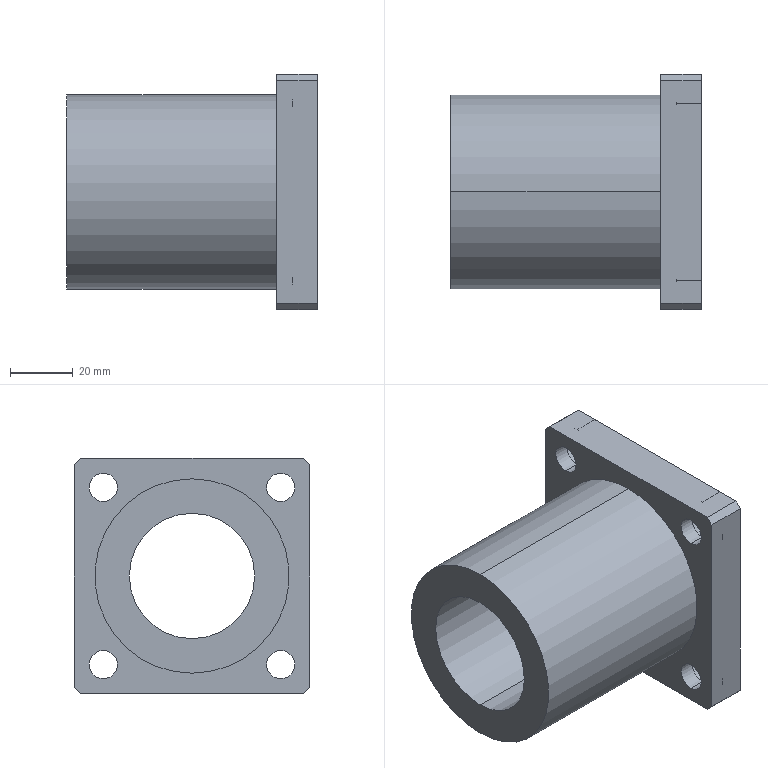Part | SolidWorks | features Chamfer 1, Extrusion 1, HoleWzd 1, ICE 1 | 1 solid | 35 faces | box 80 x 75 x 75 mm | volume 165352 mm3 | cylinder 20 | plane 15 | commonest cylinder face diameters 9 x8 18 x8 40 x2 62 x2
STEP:
#1=CARTESIAN_POINT('',(72.,28.284,-19.284));
#2=VERTEX_POINT('',#1);
#3=CARTESIAN_POINT('',(72.,28.284,-37.284));
#4=VERTEX_POINT('',#3);
#5=CARTESIAN_POINT('',(72.,28.284,-28.284));
#6=DIRECTION('',(1.,0.,0.));
#7=DIRECTION('',(0.,0.,-1.));
#8=AXIS2_PLACEMENT_3D('',#5,#6,#7);
#9=CIRCLE('',#8,9.);
#10=EDGE_CURVE('',#2,#4,#9,.T.);
#11=ORIENTED_EDGE('',*,*,#10,.F.);
#12=CARTESIAN_POINT('',(80.,28.284,-19.284));
#13=VERTEX_POINT('',#12);
#14=CARTESIAN_POINT('',(80.,28.284,-19.284));
#15=DIRECTION('',(1.,0.,0.));
#16=VECTOR('',#15,1000.);
#17=LINE('',#14,#16);
#18=EDGE_CURVE('',#2,#13,#17,.T.);
#19=ORIENTED_EDGE('',*,*,#18,.T.);
#20=CARTESIAN_POINT('',(80.,28.284,-37.284));
#21=VERTEX_POINT('',#20);
#22=CARTESIAN_POINT('',(80.,28.284,-28.284));
#23=DIRECTION('',(1.,0.,0.));
#24=DIRECTION('',(0.,0.,-1.));
#25=AXIS2_PLACEMENT_3D('',#22,#23,#24);
#26=CIRCLE('',#25,9.);
#27=EDGE_CURVE('',#13,#21,#26,.T.);
#28=ORIENTED_EDGE('',*,*,#27,.T.);
#29=CARTESIAN_POINT('',(80.,28.284,-37.284));
#30=DIRECTION('',(1.,0.,0.));
#31=VECTOR('',#30,1000.);
#32=LINE('',#29,#31);
#33=EDGE_CURVE('',#4,#21,#32,.T.);
#34=ORIENTED_EDGE('',*,*,#33,.F.);
#35=EDGE_LOOP('',(#11,#19,#28,#34));
#36=FACE_OUTER_BOUND('',#35,.T.);
#37=CARTESIAN_POINT('',(80.,28.284,-28.284));
#38=DIRECTION('',(1.,0.,0.));
#39=DIRECTION('',(0.,0.,-1.));
#40=AXIS2_PLACEMENT_3D('',#37,#38,#39);
#41=CYLINDRICAL_SURFACE('',#40,9.);
#42=ADVANCED_FACE('',(#36),#41,.F.);
#43=CARTESIAN_POINT('',(67.,28.284,-23.784));
#44=VERTEX_POINT('',#43);
#45=CARTESIAN_POINT('',(67.,28.284,-32.784));
#46=VERTEX_POINT('',#45);
#47=CARTESIAN_POINT('',(67.,28.284,-28.284));
#48=DIRECTION('',(1.,0.,0.));
#49=DIRECTION('',(0.,0.,-1.));
#50=AXIS2_PLACEMENT_3D('',#47,#48,#49);
#51=CIRCLE('',#50,4.5);
#52=EDGE_CURVE('',#44,#46,#51,.T.);
#53=ORIENTED_EDGE('',*,*,#52,.F.);
#54=CARTESIAN_POINT('',(72.,28.284,-23.784));
#55=VERTEX_POINT('',#54);
#56=CARTESIAN_POINT('',(80.,28.284,-23.784));
#57=DIRECTION('',(1.,0.,0.));
#58=VECTOR('',#57,1000.);
#59=LINE('',#56,#58);
#60=EDGE_CURVE('',#44,#55,#59,.T.);
#61=ORIENTED_EDGE('',*,*,#60,.T.);
#62=CARTESIAN_POINT('',(72.,28.284,-32.784));
#63=VERTEX_POINT('',#62);
#64=CARTESIAN_POINT('',(72.,28.284,-28.284));
#65=DIRECTION('',(1.,0.,0.));
#66=DIRECTION('',(0.,0.,-1.));
#67=AXIS2_PLACEMENT_3D('',#64,#65,#66);
#68=CIRCLE('',#67,4.5);
#69=EDGE_CURVE('',#55,#63,#68,.T.);
#70=ORIENTED_EDGE('',*,*,#69,.T.);
#71=CARTESIAN_POINT('',(80.,28.284,-32.784));
#72=DIRECTION('',(1.,0.,0.));
#73=VECTOR('',#72,1000.);
#74=LINE('',#71,#73);
#75=EDGE_CURVE('',#46,#63,#74,.T.);
#76=ORIENTED_EDGE('',*,*,#75,.F.);
#77=EDGE_LOOP('',(#53,#61,#70,#76));
#78=FACE_OUTER_BOUND('',#77,.T.);
#79=CARTESIAN_POINT('',(80.,28.284,-28.284));
#80=DIRECTION('',(1.,0.,0.));
#81=DIRECTION('',(0.,0.,-1.));
#82=AXIS2_PLACEMENT_3D('',#79,#80,#81);
#83=CYLINDRICAL_SURFACE('',#82,4.5);
#84=ADVANCED_FACE('',(#78),#83,.F.);
#85=CARTESIAN_POINT('',(72.,-28.284,-19.284));
#86=VERTEX_POINT('',#85);
#87=CARTESIAN_POINT('',(72.,-28.284,-37.284));
#88=VERTEX_POINT('',#87);
#89=CARTESIAN_POINT('',(72.,-28.284,-28.284));
#90=DIRECTION('',(1.,0.,0.));
#91=DIRECTION('',(0.,0.,-1.));
#92=AXIS2_PLACEMENT_3D('',#89,#90,#91);
#93=CIRCLE('',#92,9.);
#94=EDGE_CURVE('',#86,#88,#93,.T.);
#95=ORIENTED_EDGE('',*,*,#94,.F.);
#96=CARTESIAN_POINT('',(80.,-28.284,-19.284));
#97=VERTEX_POINT('',#96);
#98=CARTESIAN_POINT('',(80.,-28.284,-19.284));
#99=DIRECTION('',(1.,0.,0.));
#100=VECTOR('',#99,1000.);
#101=LINE('',#98,#100);
#102=EDGE_CURVE('',#86,#97,#101,.T.);
#103=ORIENTED_EDGE('',*,*,#102,.T.);
#104=CARTESIAN_POINT('',(80.,-28.284,-37.284));
#105=VERTEX_POINT('',#104);
#106=CARTESIAN_POINT('',(80.,-28.284,-28.284));
#107=DIRECTION('',(1.,0.,0.));
#108=DIRECTION('',(0.,0.,-1.));
#109=AXIS2_PLACEMENT_3D('',#106,#107,#108);
#110=CIRCLE('',#109,9.);
#111=EDGE_CURVE('',#97,#105,#110,.T.);
#112=ORIENTED_EDGE('',*,*,#111,.T.);
#113=CARTESIAN_POINT('',(80.,-28.284,-37.284));
#114=DIRECTION('',(1.,0.,0.));
#115=VECTOR('',#114,1000.);
#116=LINE('',#113,#115);
#117=EDGE_CURVE('',#88,#105,#116,.T.);
#118=ORIENTED_EDGE('',*,*,#117,.F.);
#119=EDGE_LOOP('',(#95,#103,#112,#118));
#120=FACE_OUTER_BOUND('',#119,.T.);
#121=CARTESIAN_POINT('',(80.,-28.284,-28.284));
#122=DIRECTION('',(1.,0.,0.));
#123=DIRECTION('',(0.,0.,-1.));
#124=AXIS2_PLACEMENT_3D('',#121,#122,#123);
#125=CYLINDRICAL_SURFACE('',#124,9.);
#126=ADVANCED_FACE('',(#120),#125,.F.);
#127=CARTESIAN_POINT('',(67.,-28.284,-23.784));
#128=VERTEX_POINT('',#127);
#129=CARTESIAN_POINT('',(67.,-28.284,-32.784));
#130=VERTEX_POINT('',#129);
#131=CARTESIAN_POINT('',(67.,-28.284,-28.284));
#132=DIRECTION('',(1.,0.,0.));
#133=DIRECTION('',(0.,0.,-1.));
#134=AXIS2_PLACEMENT_3D('',#131,#132,#133);
#135=CIRCLE('',#134,4.5);
#136=EDGE_CURVE('',#128,#130,#135,.T.);
#137=ORIENTED_EDGE('',*,*,#136,.F.);
#138=CARTESIAN_POINT('',(72.,-28.284,-23.784));
#139=VERTEX_POINT('',#138);
#140=CARTESIAN_POINT('',(80.,-28.284,-23.784));
#141=DIRECTION('',(1.,0.,0.));
#142=VECTOR('',#141,1000.);
#143=LINE('',#140,#142);
#144=EDGE_CURVE('',#128,#139,#143,.T.);
#145=ORIENTED_EDGE('',*,*,#144,.T.);
#146=CARTESIAN_POINT('',(72.,-28.284,-32.784));
#147=VERTEX_POINT('',#146);
#148=CARTESIAN_POINT('',(72.,-28.284,-28.284));
#149=DIRECTION('',(1.,0.,0.));
#150=DIRECTION('',(0.,0.,-1.));
#151=AXIS2_PLACEMENT_3D('',#148,#149,#150);
#152=CIRCLE('',#151,4.5);
#153=EDGE_CURVE('',#139,#147,#152,.T.);
#154=ORIENTED_EDGE('',*,*,#153,.T.);
#155=CARTESIAN_POINT('',(80.,-28.284,-32.784));
#156=DIRECTION('',(1.,0.,0.));
#157=VECTOR('',#156,1000.);
#158=LINE('',#155,#157);
#159=EDGE_CURVE('',#130,#147,#158,.T.);
#160=ORIENTED_EDGE('',*,*,#159,.F.);
#161=EDGE_LOOP('',(#137,#145,#154,#160));
#162=FACE_OUTER_BOUND('',#161,.T.);
#163=CARTESIAN_POINT('',(80.,-28.284,-28.284));
#164=DIRECTION('',(1.,0.,0.));
#165=DIRECTION('',(0.,0.,-1.));
#166=AXIS2_PLACEMENT_3D('',#163,#164,#165);
#167=CYLINDRICAL_SURFACE('',#166,4.5);
#168=ADVANCED_FACE('',(#162),#167,.F.);
#169=CARTESIAN_POINT('',(72.,-28.284,37.284));
#170=VERTEX_POINT('',#169);
#171=CARTESIAN_POINT('',(72.,-28.284,19.284));
#172=VERTEX_POINT('',#171);
#173=CARTESIAN_POINT('',(72.,-28.284,28.284));
#174=DIRECTION('',(1.,0.,0.));
#175=DIRECTION('',(0.,0.,-1.));
#176=AXIS2_PLACEMENT_3D('',#173,#174,#175);
#177=CIRCLE('',#176,9.);
#178=EDGE_CURVE('',#170,#172,#177,.T.);
#179=ORIENTED_EDGE('',*,*,#178,.F.);
#180=CARTESIAN_POINT('',(80.,-28.284,37.284));
#181=VERTEX_POINT('',#180);
#182=CARTESIAN_POINT('',(80.,-28.284,37.284));
#183=DIRECTION('',(1.,0.,0.));
#184=VECTOR('',#183,1000.);
#185=LINE('',#182,#184);
#186=EDGE_CURVE('',#170,#181,#185,.T.);
#187=ORIENTED_EDGE('',*,*,#186,.T.);
#188=CARTESIAN_POINT('',(80.,-28.284,19.284));
#189=VERTEX_POINT('',#188);
#190=CARTESIAN_POINT('',(80.,-28.284,28.284));
#191=DIRECTION('',(1.,0.,0.));
#192=DIRECTION('',(0.,0.,-1.));
#193=AXIS2_PLACEMENT_3D('',#190,#191,#192);
#194=CIRCLE('',#193,9.);
#195=EDGE_CURVE('',#181,#189,#194,.T.);
#196=ORIENTED_EDGE('',*,*,#195,.T.);
#197=CARTESIAN_POINT('',(80.,-28.284,19.284));
#198=DIRECTION('',(1.,0.,0.));
#199=VECTOR('',#198,1000.);
#200=LINE('',#197,#199);
#201=EDGE_CURVE('',#172,#189,#200,.T.);
#202=ORIENTED_EDGE('',*,*,#201,.F.);
#203=EDGE_LOOP('',(#179,#187,#196,#202));
#204=FACE_OUTER_BOUND('',#203,.T.);
#205=CARTESIAN_POINT('',(80.,-28.284,28.284));
#206=DIRECTION('',(1.,0.,0.));
#207=DIRECTION('',(0.,0.,-1.));
#208=AXIS2_PLACEMENT_3D('',#205,#206,#207);
#209=CYLINDRICAL_SURFACE('',#208,9.);
#210=ADVANCED_FACE('',(#204),#209,.F.);
#211=CARTESIAN_POINT('',(67.,-28.284,32.784));
#212=VERTEX_POINT('',#211);
#213=CARTESIAN_POINT('',(67.,-28.284,23.784));
#214=VERTEX_POINT('',#213);
#215=CARTESIAN_POINT('',(67.,-28.284,28.284));
#216=DIRECTION('',(1.,0.,0.));
#217=DIRECTION('',(0.,0.,-1.));
#218=AXIS2_PLACEMENT_3D('',#215,#216,#217);
#219=CIRCLE('',#218,4.5);
#220=EDGE_CURVE('',#212,#214,#219,.T.);
#221=ORIENTED_EDGE('',*,*,#220,.F.);
#222=CARTESIAN_POINT('',(72.,-28.284,32.784));
#223=VERTEX_POINT('',#222);
#224=CARTESIAN_POINT('',(80.,-28.284,32.784));
#225=DIRECTION('',(1.,0.,0.));
#226=VECTOR('',#225,1000.);
#227=LINE('',#224,#226);
#228=EDGE_CURVE('',#212,#223,#227,.T.);
#229=ORIENTED_EDGE('',*,*,#228,.T.);
#230=CARTESIAN_POINT('',(72.,-28.284,23.784));
#231=VERTEX_POINT('',#230);
#232=CARTESIAN_POINT('',(72.,-28.284,28.284));
#233=DIRECTION('',(1.,0.,0.));
#234=DIRECTION('',(0.,0.,-1.));
#235=AXIS2_PLACEMENT_3D('',#232,#233,#234);
#236=CIRCLE('',#235,4.5);
#237=EDGE_CURVE('',#223,#231,#236,.T.);
#238=ORIENTED_EDGE('',*,*,#237,.T.);
#239=CARTESIAN_POINT('',(80.,-28.284,23.784));
#240=DIRECTION('',(1.,0.,0.));
#241=VECTOR('',#240,1000.);
#242=LINE('',#239,#241);
#243=EDGE_CURVE('',#214,#231,#242,.T.);
#244=ORIENTED_EDGE('',*,*,#243,.F.);
#245=EDGE_LOOP('',(#221,#229,#238,#244));
#246=FACE_OUTER_BOUND('',#245,.T.);
#247=CARTESIAN_POINT('',(80.,-28.284,28.284));
#248=DIRECTION('',(1.,0.,0.));
#249=DIRECTION('',(0.,0.,-1.));
#250=AXIS2_PLACEMENT_3D('',#247,#248,#249);
#251=CYLINDRICAL_SURFACE('',#250,4.5);
#252=ADVANCED_FACE('',(#246),#251,.F.);
#253=CARTESIAN_POINT('',(72.,28.284,37.284));
#254=VERTEX_POINT('',#253);
#255=CARTESIAN_POINT('',(72.,28.284,19.284));
#256=VERTEX_POINT('',#255);
#257=CARTESIAN_POINT('',(72.,28.284,28.284));
#258=DIRECTION('',(1.,0.,0.));
#259=DIRECTION('',(0.,0.,-1.));
#260=AXIS2_PLACEMENT_3D('',#257,#258,#259);
#261=CIRCLE('',#260,9.);
#262=EDGE_CURVE('',#254,#256,#261,.T.);
#263=ORIENTED_EDGE('',*,*,#262,.F.);
#264=CARTESIAN_POINT('',(80.,28.284,37.284));
#265=VERTEX_POINT('',#264);
#266=CARTESIAN_POINT('',(80.,28.284,37.284));
#267=DIRECTION('',(1.,0.,0.));
#268=VECTOR('',#267,1000.);
#269=LINE('',#266,#268);
#270=EDGE_CURVE('',#254,#265,#269,.T.);
#271=ORIENTED_EDGE('',*,*,#270,.T.);
#272=CARTESIAN_POINT('',(80.,28.284,19.284));
#273=VERTEX_POINT('',#272);
#274=CARTESIAN_POINT('',(80.,28.284,28.284));
#275=DIRECTION('',(1.,0.,0.));
#276=DIRECTION('',(0.,0.,-1.));
#277=AXIS2_PLACEMENT_3D('',#274,#275,#276);
#278=CIRCLE('',#277,9.);
#279=EDGE_CURVE('',#265,#273,#278,.T.);
#280=ORIENTED_EDGE('',*,*,#279,.T.);
#281=CARTESIAN_POINT('',(80.,28.284,19.284));
#282=DIRECTION('',(1.,0.,0.));
#283=VECTOR('',#282,1000.);
#284=LINE('',#281,#283);
#285=EDGE_CURVE('',#256,#273,#284,.T.);
#286=ORIENTED_EDGE('',*,*,#285,.F.);
#287=EDGE_LOOP('',(#263,#271,#280,#286));
#288=FACE_OUTER_BOUND('',#287,.T.);
#289=CARTESIAN_POINT('',(80.,28.284,28.284));
#290=DIRECTION('',(1.,0.,0.));
#291=DIRECTION('',(0.,0.,-1.));
#292=AXIS2_PLACEMENT_3D('',#289,#290,#291);
#293=CYLINDRICAL_SURFACE('',#292,9.);
#294=ADVANCED_FACE('',(#288),#293,.F.);
#295=CARTESIAN_POINT('',(67.,28.284,32.784));
#296=VERTEX_POINT('',#295);
#297=CARTESIAN_POINT('',(67.,28.284,23.784));
#298=VERTEX_POINT('',#297);
#299=CARTESIAN_POINT('',(67.,28.284,28.284));
#300=DIRECTION('',(1.,0.,0.));
#301=DIRECTION('',(0.,0.,-1.));
#302=AXIS2_PLACEMENT_3D('',#299,#300,#301);
#303=CIRCLE('',#302,4.5);
#304=EDGE_CURVE('',#296,#298,#303,.T.);
#305=ORIENTED_EDGE('',*,*,#304,.F.);
#306=CARTESIAN_POINT('',(72.,28.284,32.784));
#307=VERTEX_POINT('',#306);
#308=CARTESIAN_POINT('',(80.,28.284,32.784));
#309=DIRECTION('',(1.,0.,0.));
#310=VECTOR('',#309,1000.);
#311=LINE('',#308,#310);
#312=EDGE_CURVE('',#296,#307,#311,.T.);
#313=ORIENTED_EDGE('',*,*,#312,.T.);
#314=CARTESIAN_POINT('',(72.,28.284,23.784));
#315=VERTEX_POINT('',#314);
#316=CARTESIAN_POINT('',(72.,28.284,28.284));
#317=DIRECTION('',(1.,0.,0.));
#318=DIRECTION('',(0.,0.,-1.));
#319=AXIS2_PLACEMENT_3D('',#316,#317,#318);
#320=CIRCLE('',#319,4.5);
#321=EDGE_CURVE('',#307,#315,#320,.T.);
#322=ORIENTED_EDGE('',*,*,#321,.T.);
#323=CARTESIAN_POINT('',(80.,28.284,23.784));
#324=DIRECTION('',(1.,0.,0.));
#325=VECTOR('',#324,1000.);
#326=LINE('',#323,#325);
#327=EDGE_CURVE('',#298,#315,#326,.T.);
#328=ORIENTED_EDGE('',*,*,#327,.F.);
#329=EDGE_LOOP('',(#305,#313,#322,#328));
#330=FACE_OUTER_BOUND('',#329,.T.);
#331=CARTESIAN_POINT('',(80.,28.284,28.284));
#332=DIRECTION('',(1.,0.,0.));
#333=DIRECTION('',(0.,0.,-1.));
#334=AXIS2_PLACEMENT_3D('',#331,#332,#333);
#335=CYLINDRICAL_SURFACE('',#334,4.5);
#336=ADVANCED_FACE('',(#330),#335,.F.);
#337=CARTESIAN_POINT('',(80.,0.,20.));
#338=VERTEX_POINT('',#337);
#339=CARTESIAN_POINT('',(80.,0.,-20.));
#340=VERTEX_POINT('',#339);
#341=CARTESIAN_POINT('',(80.,0.,0.));
#342=DIRECTION('',(1.,0.,0.));
#343=DIRECTION('',(0.,0.,-1.));
#344=AXIS2_PLACEMENT_3D('',#341,#342,#343);
#345=CIRCLE('',#344,20.);
#346=EDGE_CURVE('',#338,#340,#345,.T.);
#347=ORIENTED_EDGE('',*,*,#346,.T.);
#348=CARTESIAN_POINT('',(0.,0.,-20.));
#349=VERTEX_POINT('',#348);
#350=CARTESIAN_POINT('',(67.,0.,-20.));
#351=DIRECTION('',(-1.,0.,0.));
#352=VECTOR('',#351,1000.);
#353=LINE('',#350,#352);
#354=EDGE_CURVE('',#340,#349,#353,.T.);
#355=ORIENTED_EDGE('',*,*,#354,.T.);
#356=CARTESIAN_POINT('',(0.,0.,20.));
#357=VERTEX_POINT('',#356);
#358=CARTESIAN_POINT('',(0.,0.,0.));
#359=DIRECTION('',(1.,0.,0.));
#360=DIRECTION('',(0.,0.,-1.));
#361=AXIS2_PLACEMENT_3D('',#358,#359,#360);
#362=CIRCLE('',#361,20.);
#363=EDGE_CURVE('',#357,#349,#362,.T.);
#364=ORIENTED_EDGE('',*,*,#363,.F.);
#365=CARTESIAN_POINT('',(67.,0.,20.));
#366=DIRECTION('',(-1.,0.,0.));
#367=VECTOR('',#366,1000.);
#368=LINE('',#365,#367);
#369=EDGE_CURVE('',#338,#357,#368,.T.);
#370=ORIENTED_EDGE('',*,*,#369,.F.);
#371=EDGE_LOOP('',(#347,#355,#364,#370));
#372=FACE_OUTER_BOUND('',#371,.T.);
#373=CARTESIAN_POINT('',(67.,0.,0.));
#374=DIRECTION('',(-1.,0.,0.));
#375=DIRECTION('',(0.,0.,1.));
#376=AXIS2_PLACEMENT_3D('',#373,#374,#375);
#377=CYLINDRICAL_SURFACE('',#376,20.);
#378=ADVANCED_FACE('',(#372),#377,.F.);
#379=CARTESIAN_POINT('',(67.,0.,-31.));
#380=VERTEX_POINT('',#379);
#381=CARTESIAN_POINT('',(67.,0.,31.));
#382=VERTEX_POINT('',#381);
#383=CARTESIAN_POINT('',(67.,0.,0.));
#384=DIRECTION('',(1.,0.,0.));
#385=DIRECTION('',(0.,0.,-1.));
#386=AXIS2_PLACEMENT_3D('',#383,#384,#385);
#387=CIRCLE('',#386,31.);
#388=EDGE_CURVE('',#380,#382,#387,.T.);
#389=ORIENTED_EDGE('',*,*,#388,.F.);
#390=CARTESIAN_POINT('',(0.,0.,-31.));
#391=VERTEX_POINT('',#390);
#392=CARTESIAN_POINT('',(67.,0.,-31.));
#393=DIRECTION('',(-1.,0.,0.));
#394=VECTOR('',#393,1000.);
#395=LINE('',#392,#394);
#396=EDGE_CURVE('',#380,#391,#395,.T.);
#397=ORIENTED_EDGE('',*,*,#396,.T.);
#398=CARTESIAN_POINT('',(0.,0.,31.));
#399=VERTEX_POINT('',#398);
#400=CARTESIAN_POINT('',(0.,0.,0.));
#401=DIRECTION('',(1.,0.,0.));
#402=DIRECTION('',(0.,0.,-1.));
#403=AXIS2_PLACEMENT_3D('',#400,#401,#402);
#404=CIRCLE('',#403,31.);
#405=EDGE_CURVE('',#391,#399,#404,.T.);
#406=ORIENTED_EDGE('',*,*,#405,.T.);
#407=CARTESIAN_POINT('',(67.,0.,31.));
#408=DIRECTION('',(-1.,0.,0.));
#409=VECTOR('',#408,1000.);
#410=LINE('',#407,#409);
#411=EDGE_CURVE('',#382,#399,#410,.T.);
#412=ORIENTED_EDGE('',*,*,#411,.F.);
#413=EDGE_LOOP('',(#389,#397,#406,#412));
#414=FACE_OUTER_BOUND('',#413,.T.);
#415=CARTESIAN_POINT('',(67.,0.,0.));
#416=DIRECTION('',(-1.,0.,0.));
#417=DIRECTION('',(0.,0.,1.));
#418=AXIS2_PLACEMENT_3D('',#415,#416,#417);
#419=CYLINDRICAL_SURFACE('',#418,31.);
#420=ADVANCED_FACE('',(#414),#419,.T.);
#421=CARTESIAN_POINT('',(0.,0.,0.));
#422=DIRECTION('',(1.,0.,0.));
#423=DIRECTION('',(0.,0.,-1.));
#424=AXIS2_PLACEMENT_3D('',#421,#422,#423);
#425=CIRCLE('',#424,31.);
#426=EDGE_CURVE('',#399,#391,#425,.T.);
#427=ORIENTED_EDGE('',*,*,#426,.F.);
#428=ORIENTED_EDGE('',*,*,#405,.F.);
#429=EDGE_LOOP('',(#427,#428));
#430=FACE_OUTER_BOUND('',#429,.T.);
#431=ORIENTED_EDGE('',*,*,#363,.T.);
#432=CARTESIAN_POINT('',(0.,0.,0.));
#433=DIRECTION('',(1.,0.,0.));
#434=DIRECTION('',(0.,0.,-1.));
#435=AXIS2_PLACEMENT_3D('',#432,#433,#434);
#436=CIRCLE('',#435,20.);
#437=EDGE_CURVE('',#349,#357,#436,.T.);
#438=ORIENTED_EDGE('',*,*,#437,.T.);
#439=EDGE_LOOP('',(#431,#438));
#440=FACE_BOUND('',#439,.T.);
#441=CARTESIAN_POINT('',(0.,0.,0.));
#442=DIRECTION('',(1.,0.,0.));
#443=DIRECTION('',(0.,0.,-1.));
#444=AXIS2_PLACEMENT_3D('',#441,#442,#443);
#445=PLANE('',#444);
#446=ADVANCED_FACE('',(#430,#440),#445,.F.);
#447=ORIENTED_EDGE('',*,*,#396,.F.);
#448=CARTESIAN_POINT('',(67.,0.,0.));
#449=DIRECTION('',(1.,0.,0.));
#450=DIRECTION('',(0.,0.,-1.));
#451=AXIS2_PLACEMENT_3D('',#448,#449,#450);
#452=CIRCLE('',#451,31.);
#453=EDGE_CURVE('',#382,#380,#452,.T.);
#454=ORIENTED_EDGE('',*,*,#453,.F.);
#455=ORIENTED_EDGE('',*,*,#411,.T.);
#456=ORIENTED_EDGE('',*,*,#426,.T.);
#457=EDGE_LOOP('',(#447,#454,#455,#456));
#458=FACE_OUTER_BOUND('',#457,.T.);
#459=CARTESIAN_POINT('',(67.,0.,0.));
#460=DIRECTION('',(-1.,0.,0.));
#461=DIRECTION('',(0.,0.,1.));
#462=AXIS2_PLACEMENT_3D('',#459,#460,#461);
#463=CYLINDRICAL_SURFACE('',#462,31.);
#464=ADVANCED_FACE('',(#458),#463,.T.);
#465=ORIENTED_EDGE('',*,*,#354,.F.);
#466=CARTESIAN_POINT('',(80.,0.,0.));
#467=DIRECTION('',(1.,0.,0.));
#468=DIRECTION('',(0.,0.,-1.));
#469=AXIS2_PLACEMENT_3D('',#466,#467,#468);
#470=CIRCLE('',#469,20.);
#471=EDGE_CURVE('',#340,#338,#470,.T.);
#472=ORIENTED_EDGE('',*,*,#471,.T.);
#473=ORIENTED_EDGE('',*,*,#369,.T.);
#474=ORIENTED_EDGE('',*,*,#437,.F.);
#475=EDGE_LOOP('',(#465,#472,#473,#474));
#476=FACE_OUTER_BOUND('',#475,.T.);
#477=CARTESIAN_POINT('',(67.,0.,0.));
#478=DIRECTION('',(-1.,0.,0.));
#479=DIRECTION('',(0.,0.,1.));
#480=AXIS2_PLACEMENT_3D('',#477,#478,#479);
#481=CYLINDRICAL_SURFACE('',#480,20.);
#482=ADVANCED_FACE('',(#476),#481,.F.);
#483=CARTESIAN_POINT('',(67.,28.284,-28.284));
#484=DIRECTION('',(1.,0.,0.));
#485=DIRECTION('',(0.,0.,-1.));
#486=AXIS2_PLACEMENT_3D('',#483,#484,#485);
#487=CIRCLE('',#486,4.5);
#488=EDGE_CURVE('',#46,#44,#487,.T.);
#489=ORIENTED_EDGE('',*,*,#488,.T.);
#490=ORIENTED_EDGE('',*,*,#52,.T.);
#491=EDGE_LOOP('',(#489,#490));
#492=FACE_BOUND('',#491,.T.);
#493=CARTESIAN_POINT('',(67.,-28.284,-28.284));
#494=DIRECTION('',(1.,0.,0.));
#495=DIRECTION('',(0.,0.,-1.));
#496=AXIS2_PLACEMENT_3D('',#493,#494,#495);
#497=CIRCLE('',#496,4.5);
#498=EDGE_CURVE('',#130,#128,#497,.T.);
#499=ORIENTED_EDGE('',*,*,#498,.T.);
#500=ORIENTED_EDGE('',*,*,#136,.T.);
#501=EDGE_LOOP('',(#499,#500));
#502=FACE_BOUND('',#501,.T.);
#503=CARTESIAN_POINT('',(67.,-28.284,28.284));
#504=DIRECTION('',(1.,0.,0.));
#505=DIRECTION('',(0.,0.,-1.));
#506=AXIS2_PLACEMENT_3D('',#503,#504,#505);
#507=CIRCLE('',#506,4.5);
#508=EDGE_CURVE('',#214,#212,#507,.T.);
#509=ORIENTED_EDGE('',*,*,#508,.T.);
#510=ORIENTED_EDGE('',*,*,#220,.T.);
#511=EDGE_LOOP('',(#509,#510));
#512=FACE_BOUND('',#511,.T.);
#513=CARTESIAN_POINT('',(67.,28.284,28.284));
#514=DIRECTION('',(1.,0.,0.));
#515=DIRECTION('',(0.,0.,-1.));
#516=AXIS2_PLACEMENT_3D('',#513,#514,#515);
#517=CIRCLE('',#516,4.5);
#518=EDGE_CURVE('',#298,#296,#517,.T.);
#519=ORIENTED_EDGE('',*,*,#518,.T.);
#520=ORIENTED_EDGE('',*,*,#304,.T.);
#521=EDGE_LOOP('',(#519,#520));
#522=FACE_BOUND('',#521,.T.);
#523=CARTESIAN_POINT('',(67.,35.5,37.5));
#524=VERTEX_POINT('',#523);
#525=CARTESIAN_POINT('',(67.,-35.5,37.5));
#526=VERTEX_POINT('',#525);
#527=CARTESIAN_POINT('',(67.,37.5,37.5));
#528=DIRECTION('',(0.,-1.,0.));
#529=VECTOR('',#528,1000.);
#530=LINE('',#527,#529);
#531=EDGE_CURVE('',#524,#526,#530,.T.);
#532=ORIENTED_EDGE('',*,*,#531,.F.);
#533=CARTESIAN_POINT('',(67.,37.5,35.5));
#534=VERTEX_POINT('',#533);
#535=CARTESIAN_POINT('',(67.,35.5,37.5));
#536=DIRECTION('',(0.,0.7071,-0.7071));
#537=VECTOR('',#536,1000.);
#538=LINE('',#535,#537);
#539=EDGE_CURVE('',#524,#534,#538,.T.);
#540=ORIENTED_EDGE('',*,*,#539,.T.);
#541=CARTESIAN_POINT('',(67.,37.5,-35.5));
#542=VERTEX_POINT('',#541);
#543=CARTESIAN_POINT('',(67.,37.5,37.5));
#544=DIRECTION('',(0.,0.,1.));
#545=VECTOR('',#544,1000.);
#546=LINE('',#543,#545);
#547=EDGE_CURVE('',#542,#534,#546,.T.);
#548=ORIENTED_EDGE('',*,*,#547,.F.);
#549=CARTESIAN_POINT('',(67.,35.5,-37.5));
#550=VERTEX_POINT('',#549);
#551=CARTESIAN_POINT('',(67.,37.5,-35.5));
#552=DIRECTION('',(0.,-0.7071,-0.7071));
#553=VECTOR('',#552,1000.);
#554=LINE('',#551,#553);
#555=EDGE_CURVE('',#542,#550,#554,.T.);
#556=ORIENTED_EDGE('',*,*,#555,.T.);
#557=CARTESIAN_POINT('',(67.,-35.5,-37.5));
#558=VERTEX_POINT('',#557);
#559=CARTESIAN_POINT('',(67.,37.5,-37.5));
#560=DIRECTION('',(0.,1.,0.));
#561=VECTOR('',#560,1000.);
#562=LINE('',#559,#561);
#563=EDGE_CURVE('',#558,#550,#562,.T.);
#564=ORIENTED_EDGE('',*,*,#563,.F.);
#565=CARTESIAN_POINT('',(67.,-37.5,-35.5));
#566=VERTEX_POINT('',#565);
#567=CARTESIAN_POINT('',(67.,-35.5,-37.5));
#568=DIRECTION('',(0.,-0.7071,0.7071));
#569=VECTOR('',#568,1000.);
#570=LINE('',#567,#569);
#571=EDGE_CURVE('',#558,#566,#570,.T.);
#572=ORIENTED_EDGE('',*,*,#571,.T.);
#573=CARTESIAN_POINT('',(67.,-37.5,35.5));
#574=VERTEX_POINT('',#573);
#575=CARTESIAN_POINT('',(67.,-37.5,37.5));
#576=DIRECTION('',(0.,0.,-1.));
#577=VECTOR('',#576,1000.);
#578=LINE('',#575,#577);
#579=EDGE_CURVE('',#574,#566,#578,.T.);
#580=ORIENTED_EDGE('',*,*,#579,.F.);
#581=CARTESIAN_POINT('',(67.,-37.5,35.5));
#582=DIRECTION('',(0.,0.7071,0.7071));
#583=VECTOR('',#582,1000.);
#584=LINE('',#581,#583);
#585=EDGE_CURVE('',#574,#526,#584,.T.);
#586=ORIENTED_EDGE('',*,*,#585,.T.);
#587=EDGE_LOOP('',(#532,#540,#548,#556,#564,#572,#580,#586));
#588=FACE_OUTER_BOUND('',#587,.T.);
#589=ORIENTED_EDGE('',*,*,#453,.T.);
#590=ORIENTED_EDGE('',*,*,#388,.T.);
#591=EDGE_LOOP('',(#589,#590));
#592=FACE_BOUND('',#591,.T.);
#593=CARTESIAN_POINT('',(67.,0.,0.));
#594=DIRECTION('',(1.,0.,0.));
#595=DIRECTION('',(0.,0.,-1.));
#596=AXIS2_PLACEMENT_3D('',#593,#594,#595);
#597=PLANE('',#596);
#598=ADVANCED_FACE('',(#492,#502,#512,#522,#588,#592),#597,.F.);
#599=CARTESIAN_POINT('',(80.,28.284,-28.284));
#600=DIRECTION('',(1.,0.,0.));
#601=DIRECTION('',(0.,0.,-1.));
#602=AXIS2_PLACEMENT_3D('',#599,#600,#601);
#603=CIRCLE('',#602,9.);
#604=EDGE_CURVE('',#21,#13,#603,.T.);
#605=ORIENTED_EDGE('',*,*,#604,.F.);
#606=ORIENTED_EDGE('',*,*,#27,.F.);
#607=EDGE_LOOP('',(#605,#606));
#608=FACE_BOUND('',#607,.T.);
#609=CARTESIAN_POINT('',(80.,-28.284,-28.284));
#610=DIRECTION('',(1.,0.,0.));
#611=DIRECTION('',(0.,0.,-1.));
#612=AXIS2_PLACEMENT_3D('',#609,#610,#611);
#613=CIRCLE('',#612,9.);
#614=EDGE_CURVE('',#105,#97,#613,.T.);
#615=ORIENTED_EDGE('',*,*,#614,.F.);
#616=ORIENTED_EDGE('',*,*,#111,.F.);
#617=EDGE_LOOP('',(#615,#616));
#618=FACE_BOUND('',#617,.T.);
#619=CARTESIAN_POINT('',(80.,-28.284,28.284));
#620=DIRECTION('',(1.,0.,0.));
#621=DIRECTION('',(0.,0.,-1.));
#622=AXIS2_PLACEMENT_3D('',#619,#620,#621);
#623=CIRCLE('',#622,9.);
#624=EDGE_CURVE('',#189,#181,#623,.T.);
#625=ORIENTED_EDGE('',*,*,#624,.F.);
#626=ORIENTED_EDGE('',*,*,#195,.F.);
#627=EDGE_LOOP('',(#625,#626));
#628=FACE_BOUND('',#627,.T.);
#629=CARTESIAN_POINT('',(80.,28.284,28.284));
#630=DIRECTION('',(1.,0.,0.));
#631=DIRECTION('',(0.,0.,-1.));
#632=AXIS2_PLACEMENT_3D('',#629,#630,#631);
#633=CIRCLE('',#632,9.);
#634=EDGE_CURVE('',#273,#265,#633,.T.);
#635=ORIENTED_EDGE('',*,*,#634,.F.);
#636=ORIENTED_EDGE('',*,*,#279,.F.);
#637=EDGE_LOOP('',(#635,#636));
#638=FACE_BOUND('',#637,.T.);
#639=CARTESIAN_POINT('',(80.,37.5,-35.5));
#640=VERTEX_POINT('',#639);
#641=CARTESIAN_POINT('',(80.,37.5,35.5));
#642=VERTEX_POINT('',#641);
#643=CARTESIAN_POINT('',(80.,37.5,37.5));
#644=DIRECTION('',(0.,0.,1.));
#645=VECTOR('',#644,1000.);
#646=LINE('',#643,#645);
#647=EDGE_CURVE('',#640,#642,#646,.T.);
#648=ORIENTED_EDGE('',*,*,#647,.T.);
#649=CARTESIAN_POINT('',(80.,35.5,37.5));
#650=VERTEX_POINT('',#649);
#651=CARTESIAN_POINT('',(80.,36.5,36.5));
#652=DIRECTION('',(0.,-0.7071,0.7071));
#653=VECTOR('',#652,1000.);
#654=LINE('',#651,#653);
#655=EDGE_CURVE('',#642,#650,#654,.T.);
#656=ORIENTED_EDGE('',*,*,#655,.T.);
#657=CARTESIAN_POINT('',(80.,-35.5,37.5));
#658=VERTEX_POINT('',#657);
#659=CARTESIAN_POINT('',(80.,37.5,37.5));
#660=DIRECTION('',(0.,-1.,0.));
#661=VECTOR('',#660,1000.);
#662=LINE('',#659,#661);
#663=EDGE_CURVE('',#650,#658,#662,.T.);
#664=ORIENTED_EDGE('',*,*,#663,.T.);
#665=CARTESIAN_POINT('',(80.,-37.5,35.5));
#666=VERTEX_POINT('',#665);
#667=CARTESIAN_POINT('',(80.,-36.5,36.5));
#668=DIRECTION('',(0.,-0.7071,-0.7071));
#669=VECTOR('',#668,1000.);
#670=LINE('',#667,#669);
#671=EDGE_CURVE('',#658,#666,#670,.T.);
#672=ORIENTED_EDGE('',*,*,#671,.T.);
#673=CARTESIAN_POINT('',(80.,-37.5,-35.5));
#674=VERTEX_POINT('',#673);
#675=CARTESIAN_POINT('',(80.,-37.5,37.5));
#676=DIRECTION('',(0.,0.,-1.));
#677=VECTOR('',#676,1000.);
#678=LINE('',#675,#677);
#679=EDGE_CURVE('',#666,#674,#678,.T.);
#680=ORIENTED_EDGE('',*,*,#679,.T.);
#681=CARTESIAN_POINT('',(80.,-35.5,-37.5));
#682=VERTEX_POINT('',#681);
#683=CARTESIAN_POINT('',(80.,-36.5,-36.5));
#684=DIRECTION('',(0.,0.7071,-0.7071));
#685=VECTOR('',#684,1000.);
#686=LINE('',#683,#685);
#687=EDGE_CURVE('',#674,#682,#686,.T.);
#688=ORIENTED_EDGE('',*,*,#687,.T.);
#689=CARTESIAN_POINT('',(80.,35.5,-37.5));
#690=VERTEX_POINT('',#689);
#691=CARTESIAN_POINT('',(80.,37.5,-37.5));
#692=DIRECTION('',(0.,1.,0.));
#693=VECTOR('',#692,1000.);
#694=LINE('',#691,#693);
#695=EDGE_CURVE('',#682,#690,#694,.T.);
#696=ORIENTED_EDGE('',*,*,#695,.T.);
#697=CARTESIAN_POINT('',(80.,36.5,-36.5));
#698=DIRECTION('',(0.,0.7071,0.7071));
#699=VECTOR('',#698,1000.);
#700=LINE('',#697,#699);
#701=EDGE_CURVE('',#690,#640,#700,.T.);
#702=ORIENTED_EDGE('',*,*,#701,.T.);
#703=EDGE_LOOP('',(#648,#656,#664,#672,#680,#688,#696,#702));
#704=FACE_OUTER_BOUND('',#703,.T.);
#705=ORIENTED_EDGE('',*,*,#346,.F.);
#706=ORIENTED_EDGE('',*,*,#471,.F.);
#707=EDGE_LOOP('',(#705,#706));
#708=FACE_BOUND('',#707,.T.);
#709=CARTESIAN_POINT('',(80.,0.,0.));
#710=DIRECTION('',(1.,0.,0.));
#711=DIRECTION('',(0.,0.,-1.));
#712=AXIS2_PLACEMENT_3D('',#709,#710,#711);
#713=PLANE('',#712);
#714=ADVANCED_FACE('',(#608,#618,#628,#638,#704,#708),#713,.T.);
#715=ORIENTED_EDGE('',*,*,#563,.T.);
#716=CARTESIAN_POINT('',(80.,35.5,-37.5));
#717=DIRECTION('',(1.,0.,0.));
#718=VECTOR('',#717,1000.);
#719=LINE('',#716,#718);
#720=EDGE_CURVE('',#550,#690,#719,.T.);
#721=ORIENTED_EDGE('',*,*,#720,.T.);
#722=ORIENTED_EDGE('',*,*,#695,.F.);
#723=CARTESIAN_POINT('',(80.,-35.5,-37.5));
#724=DIRECTION('',(-1.,0.,0.));
#725=VECTOR('',#724,1000.);
#726=LINE('',#723,#725);
#727=EDGE_CURVE('',#682,#558,#726,.T.);
#728=ORIENTED_EDGE('',*,*,#727,.T.);
#729=EDGE_LOOP('',(#715,#721,#722,#728));
#730=FACE_OUTER_BOUND('',#729,.T.);
#731=CARTESIAN_POINT('',(80.,37.5,-37.5));
#732=DIRECTION('',(0.,0.,1.));
#733=DIRECTION('',(0.,-1.,0.));
#734=AXIS2_PLACEMENT_3D('',#731,#732,#733);
#735=PLANE('',#734);
#736=ADVANCED_FACE('',(#730),#735,.F.);
#737=ORIENTED_EDGE('',*,*,#547,.T.);
#738=CARTESIAN_POINT('',(80.,37.5,35.5));
#739=DIRECTION('',(1.,0.,0.));
#740=VECTOR('',#739,1000.);
#741=LINE('',#738,#740);
#742=EDGE_CURVE('',#534,#642,#741,.T.);
#743=ORIENTED_EDGE('',*,*,#742,.T.);
#744=ORIENTED_EDGE('',*,*,#647,.F.);
#745=CARTESIAN_POINT('',(80.,37.5,-35.5));
#746=DIRECTION('',(-1.,0.,0.));
#747=VECTOR('',#746,1000.);
#748=LINE('',#745,#747);
#749=EDGE_CURVE('',#640,#542,#748,.T.);
#750=ORIENTED_EDGE('',*,*,#749,.T.);
#751=EDGE_LOOP('',(#737,#743,#744,#750));
#752=FACE_OUTER_BOUND('',#751,.T.);
#753=CARTESIAN_POINT('',(80.,37.5,37.5));
#754=DIRECTION('',(0.,-1.,0.));
#755=DIRECTION('',(0.,0.,-1.));
#756=AXIS2_PLACEMENT_3D('',#753,#754,#755);
#757=PLANE('',#756);
#758=ADVANCED_FACE('',(#752),#757,.F.);
#759=ORIENTED_EDGE('',*,*,#663,.F.);
#760=CARTESIAN_POINT('',(80.,35.5,37.5));
#761=DIRECTION('',(-1.,0.,0.));
#762=VECTOR('',#761,1000.);
#763=LINE('',#760,#762);
#764=EDGE_CURVE('',#650,#524,#763,.T.);
#765=ORIENTED_EDGE('',*,*,#764,.T.);
#766=ORIENTED_EDGE('',*,*,#531,.T.);
#767=CARTESIAN_POINT('',(80.,-35.5,37.5));
#768=DIRECTION('',(1.,0.,0.));
#769=VECTOR('',#768,1000.);
#770=LINE('',#767,#769);
#771=EDGE_CURVE('',#526,#658,#770,.T.);
#772=ORIENTED_EDGE('',*,*,#771,.T.);
#773=EDGE_LOOP('',(#759,#765,#766,#772));
#774=FACE_OUTER_BOUND('',#773,.T.);
#775=CARTESIAN_POINT('',(80.,37.5,37.5));
#776=DIRECTION('',(0.,0.,-1.));
#777=DIRECTION('',(0.,1.,0.));
#778=AXIS2_PLACEMENT_3D('',#775,#776,#777);
#779=PLANE('',#778);
#780=ADVANCED_FACE('',(#774),#779,.F.);
#781=ORIENTED_EDGE('',*,*,#579,.T.);
#782=CARTESIAN_POINT('',(80.,-37.5,-35.5));
#783=DIRECTION('',(1.,0.,0.));
#784=VECTOR('',#783,1000.);
#785=LINE('',#782,#784);
#786=EDGE_CURVE('',#566,#674,#785,.T.);
#787=ORIENTED_EDGE('',*,*,#786,.T.);
#788=ORIENTED_EDGE('',*,*,#679,.F.);
#789=CARTESIAN_POINT('',(80.,-37.5,35.5));
#790=DIRECTION('',(-1.,0.,0.));
#791=VECTOR('',#790,1000.);
#792=LINE('',#789,#791);
#793=EDGE_CURVE('',#666,#574,#792,.T.);
#794=ORIENTED_EDGE('',*,*,#793,.T.);
#795=EDGE_LOOP('',(#781,#787,#788,#794));
#796=FACE_OUTER_BOUND('',#795,.T.);
#797=CARTESIAN_POINT('',(80.,-37.5,37.5));
#798=DIRECTION('',(0.,1.,0.));
#799=DIRECTION('',(0.,0.,1.));
#800=AXIS2_PLACEMENT_3D('',#797,#798,#799);
#801=PLANE('',#800);
#802=ADVANCED_FACE('',(#796),#801,.F.);
#803=ORIENTED_EDGE('',*,*,#312,.F.);
#804=ORIENTED_EDGE('',*,*,#518,.F.);
#805=ORIENTED_EDGE('',*,*,#327,.T.);
#806=CARTESIAN_POINT('',(72.,28.284,28.284));
#807=DIRECTION('',(1.,0.,0.));
#808=DIRECTION('',(0.,0.,-1.));
#809=AXIS2_PLACEMENT_3D('',#806,#807,#808);
#810=CIRCLE('',#809,4.5);
#811=EDGE_CURVE('',#315,#307,#810,.T.);
#812=ORIENTED_EDGE('',*,*,#811,.T.);
#813=EDGE_LOOP('',(#803,#804,#805,#812));
#814=FACE_OUTER_BOUND('',#813,.T.);
#815=CARTESIAN_POINT('',(80.,28.284,28.284));
#816=DIRECTION('',(1.,0.,0.));
#817=DIRECTION('',(0.,0.,-1.));
#818=AXIS2_PLACEMENT_3D('',#815,#816,#817);
#819=CYLINDRICAL_SURFACE('',#818,4.5);
#820=ADVANCED_FACE('',(#814),#819,.F.);
#821=ORIENTED_EDGE('',*,*,#811,.F.);
#822=ORIENTED_EDGE('',*,*,#321,.F.);
#823=EDGE_LOOP('',(#821,#822));
#824=FACE_BOUND('',#823,.T.);
#825=CARTESIAN_POINT('',(72.,28.284,28.284));
#826=DIRECTION('',(1.,0.,0.));
#827=DIRECTION('',(0.,0.,-1.));
#828=AXIS2_PLACEMENT_3D('',#825,#826,#827);
#829=CIRCLE('',#828,9.);
#830=EDGE_CURVE('',#256,#254,#829,.T.);
#831=ORIENTED_EDGE('',*,*,#830,.T.);
#832=ORIENTED_EDGE('',*,*,#262,.T.);
#833=EDGE_LOOP('',(#831,#832));
#834=FACE_OUTER_BOUND('',#833,.T.);
#835=CARTESIAN_POINT('',(72.,32.784,28.284));
#836=DIRECTION('',(-1.,0.,0.));
#837=DIRECTION('',(0.,0.,1.));
#838=AXIS2_PLACEMENT_3D('',#835,#836,#837);
#839=PLANE('',#838);
#840=ADVANCED_FACE('',(#824,#834),#839,.F.);
#841=ORIENTED_EDGE('',*,*,#270,.F.);
#842=ORIENTED_EDGE('',*,*,#830,.F.);
#843=ORIENTED_EDGE('',*,*,#285,.T.);
#844=ORIENTED_EDGE('',*,*,#634,.T.);
#845=EDGE_LOOP('',(#841,#842,#843,#844));
#846=FACE_OUTER_BOUND('',#845,.T.);
#847=CARTESIAN_POINT('',(80.,28.284,28.284));
#848=DIRECTION('',(1.,0.,0.));
#849=DIRECTION('',(0.,0.,-1.));
#850=AXIS2_PLACEMENT_3D('',#847,#848,#849);
#851=CYLINDRICAL_SURFACE('',#850,9.);
#852=ADVANCED_FACE('',(#846),#851,.F.);
#853=ORIENTED_EDGE('',*,*,#228,.F.);
#854=ORIENTED_EDGE('',*,*,#508,.F.);
#855=ORIENTED_EDGE('',*,*,#243,.T.);
#856=CARTESIAN_POINT('',(72.,-28.284,28.284));
#857=DIRECTION('',(1.,0.,0.));
#858=DIRECTION('',(0.,0.,-1.));
#859=AXIS2_PLACEMENT_3D('',#856,#857,#858);
#860=CIRCLE('',#859,4.5);
#861=EDGE_CURVE('',#231,#223,#860,.T.);
#862=ORIENTED_EDGE('',*,*,#861,.T.);
#863=EDGE_LOOP('',(#853,#854,#855,#862));
#864=FACE_OUTER_BOUND('',#863,.T.);
#865=CARTESIAN_POINT('',(80.,-28.284,28.284));
#866=DIRECTION('',(1.,0.,0.));
#867=DIRECTION('',(0.,0.,-1.));
#868=AXIS2_PLACEMENT_3D('',#865,#866,#867);
#869=CYLINDRICAL_SURFACE('',#868,4.5);
#870=ADVANCED_FACE('',(#864),#869,.F.);
#871=ORIENTED_EDGE('',*,*,#861,.F.);
#872=ORIENTED_EDGE('',*,*,#237,.F.);
#873=EDGE_LOOP('',(#871,#872));
#874=FACE_BOUND('',#873,.T.);
#875=CARTESIAN_POINT('',(72.,-28.284,28.284));
#876=DIRECTION('',(1.,0.,0.));
#877=DIRECTION('',(0.,0.,-1.));
#878=AXIS2_PLACEMENT_3D('',#875,#876,#877);
#879=CIRCLE('',#878,9.);
#880=EDGE_CURVE('',#172,#170,#879,.T.);
#881=ORIENTED_EDGE('',*,*,#880,.T.);
#882=ORIENTED_EDGE('',*,*,#178,.T.);
#883=EDGE_LOOP('',(#881,#882));
#884=FACE_OUTER_BOUND('',#883,.T.);
#885=CARTESIAN_POINT('',(72.,-23.784,28.284));
#886=DIRECTION('',(-1.,0.,0.));
#887=DIRECTION('',(0.,0.,1.));
#888=AXIS2_PLACEMENT_3D('',#885,#886,#887);
#889=PLANE('',#888);
#890=ADVANCED_FACE('',(#874,#884),#889,.F.);
#891=ORIENTED_EDGE('',*,*,#186,.F.);
#892=ORIENTED_EDGE('',*,*,#880,.F.);
#893=ORIENTED_EDGE('',*,*,#201,.T.);
#894=ORIENTED_EDGE('',*,*,#624,.T.);
#895=EDGE_LOOP('',(#891,#892,#893,#894));
#896=FACE_OUTER_BOUND('',#895,.T.);
#897=CARTESIAN_POINT('',(80.,-28.284,28.284));
#898=DIRECTION('',(1.,0.,0.));
#899=DIRECTION('',(0.,0.,-1.));
#900=AXIS2_PLACEMENT_3D('',#897,#898,#899);
#901=CYLINDRICAL_SURFACE('',#900,9.);
#902=ADVANCED_FACE('',(#896),#901,.F.);
#903=ORIENTED_EDGE('',*,*,#144,.F.);
#904=ORIENTED_EDGE('',*,*,#498,.F.);
#905=ORIENTED_EDGE('',*,*,#159,.T.);
#906=CARTESIAN_POINT('',(72.,-28.284,-28.284));
#907=DIRECTION('',(1.,0.,0.));
#908=DIRECTION('',(0.,0.,-1.));
#909=AXIS2_PLACEMENT_3D('',#906,#907,#908);
#910=CIRCLE('',#909,4.5);
#911=EDGE_CURVE('',#147,#139,#910,.T.);
#912=ORIENTED_EDGE('',*,*,#911,.T.);
#913=EDGE_LOOP('',(#903,#904,#905,#912));
#914=FACE_OUTER_BOUND('',#913,.T.);
#915=CARTESIAN_POINT('',(80.,-28.284,-28.284));
#916=DIRECTION('',(1.,0.,0.));
#917=DIRECTION('',(0.,0.,-1.));
#918=AXIS2_PLACEMENT_3D('',#915,#916,#917);
#919=CYLINDRICAL_SURFACE('',#918,4.5);
#920=ADVANCED_FACE('',(#914),#919,.F.);
#921=ORIENTED_EDGE('',*,*,#911,.F.);
#922=ORIENTED_EDGE('',*,*,#153,.F.);
#923=EDGE_LOOP('',(#921,#922));
#924=FACE_BOUND('',#923,.T.);
#925=CARTESIAN_POINT('',(72.,-28.284,-28.284));
#926=DIRECTION('',(1.,0.,0.));
#927=DIRECTION('',(0.,0.,-1.));
#928=AXIS2_PLACEMENT_3D('',#925,#926,#927);
#929=CIRCLE('',#928,9.);
#930=EDGE_CURVE('',#88,#86,#929,.T.);
#931=ORIENTED_EDGE('',*,*,#930,.T.);
#932=ORIENTED_EDGE('',*,*,#94,.T.);
#933=EDGE_LOOP('',(#931,#932));
#934=FACE_OUTER_BOUND('',#933,.T.);
#935=CARTESIAN_POINT('',(72.,-23.784,-28.284));
#936=DIRECTION('',(-1.,0.,0.));
#937=DIRECTION('',(0.,0.,1.));
#938=AXIS2_PLACEMENT_3D('',#935,#936,#937);
#939=PLANE('',#938);
#940=ADVANCED_FACE('',(#924,#934),#939,.F.);
#941=ORIENTED_EDGE('',*,*,#102,.F.);
#942=ORIENTED_EDGE('',*,*,#930,.F.);
#943=ORIENTED_EDGE('',*,*,#117,.T.);
#944=ORIENTED_EDGE('',*,*,#614,.T.);
#945=EDGE_LOOP('',(#941,#942,#943,#944));
#946=FACE_OUTER_BOUND('',#945,.T.);
#947=CARTESIAN_POINT('',(80.,-28.284,-28.284));
#948=DIRECTION('',(1.,0.,0.));
#949=DIRECTION('',(0.,0.,-1.));
#950=AXIS2_PLACEMENT_3D('',#947,#948,#949);
#951=CYLINDRICAL_SURFACE('',#950,9.);
#952=ADVANCED_FACE('',(#946),#951,.F.);
#953=ORIENTED_EDGE('',*,*,#60,.F.);
#954=ORIENTED_EDGE('',*,*,#488,.F.);
#955=ORIENTED_EDGE('',*,*,#75,.T.);
#956=CARTESIAN_POINT('',(72.,28.284,-28.284));
#957=DIRECTION('',(1.,0.,0.));
#958=DIRECTION('',(0.,0.,-1.));
#959=AXIS2_PLACEMENT_3D('',#956,#957,#958);
#960=CIRCLE('',#959,4.5);
#961=EDGE_CURVE('',#63,#55,#960,.T.);
#962=ORIENTED_EDGE('',*,*,#961,.T.);
#963=EDGE_LOOP('',(#953,#954,#955,#962));
#964=FACE_OUTER_BOUND('',#963,.T.);
#965=CARTESIAN_POINT('',(80.,28.284,-28.284));
#966=DIRECTION('',(1.,0.,0.));
#967=DIRECTION('',(0.,0.,-1.));
#968=AXIS2_PLACEMENT_3D('',#965,#966,#967);
#969=CYLINDRICAL_SURFACE('',#968,4.5);
#970=ADVANCED_FACE('',(#964),#969,.F.);
#971=ORIENTED_EDGE('',*,*,#961,.F.);
#972=ORIENTED_EDGE('',*,*,#69,.F.);
#973=EDGE_LOOP('',(#971,#972));
#974=FACE_BOUND('',#973,.T.);
#975=CARTESIAN_POINT('',(72.,28.284,-28.284));
#976=DIRECTION('',(1.,0.,0.));
#977=DIRECTION('',(0.,0.,-1.));
#978=AXIS2_PLACEMENT_3D('',#975,#976,#977);
#979=CIRCLE('',#978,9.);
#980=EDGE_CURVE('',#4,#2,#979,.T.);
#981=ORIENTED_EDGE('',*,*,#980,.T.);
#982=ORIENTED_EDGE('',*,*,#10,.T.);
#983=EDGE_LOOP('',(#981,#982));
#984=FACE_OUTER_BOUND('',#983,.T.);
#985=CARTESIAN_POINT('',(72.,32.784,-28.284));
#986=DIRECTION('',(-1.,0.,0.));
#987=DIRECTION('',(0.,0.,1.));
#988=AXIS2_PLACEMENT_3D('',#985,#986,#987);
#989=PLANE('',#988);
#990=ADVANCED_FACE('',(#974,#984),#989,.F.);
#991=ORIENTED_EDGE('',*,*,#18,.F.);
#992=ORIENTED_EDGE('',*,*,#980,.F.);
#993=ORIENTED_EDGE('',*,*,#33,.T.);
#994=ORIENTED_EDGE('',*,*,#604,.T.);
#995=EDGE_LOOP('',(#991,#992,#993,#994));
#996=FACE_OUTER_BOUND('',#995,.T.);
#997=CARTESIAN_POINT('',(80.,28.284,-28.284));
#998=DIRECTION('',(1.,0.,0.));
#999=DIRECTION('',(0.,0.,-1.));
#1000=AXIS2_PLACEMENT_3D('',#997,#998,#999);
#1001=CYLINDRICAL_SURFACE('',#1000,9.);
#1002=ADVANCED_FACE('',(#996),#1001,.F.);
#1003=ORIENTED_EDGE('',*,*,#655,.F.);
#1004=ORIENTED_EDGE('',*,*,#742,.F.);
#1005=ORIENTED_EDGE('',*,*,#539,.F.);
#1006=ORIENTED_EDGE('',*,*,#764,.F.);
#1007=EDGE_LOOP('',(#1003,#1004,#1005,#1006));
#1008=FACE_OUTER_BOUND('',#1007,.T.);
#1009=CARTESIAN_POINT('',(80.,35.5,37.5));
#1010=DIRECTION('',(0.,-0.7071,-0.7071));
#1011=DIRECTION('',(-1.,0.,0.));
#1012=AXIS2_PLACEMENT_3D('',#1009,#1010,#1011);
#1013=PLANE('',#1012);
#1014=ADVANCED_FACE('',(#1008),#1013,.F.);
#1015=ORIENTED_EDGE('',*,*,#701,.F.);
#1016=ORIENTED_EDGE('',*,*,#720,.F.);
#1017=ORIENTED_EDGE('',*,*,#555,.F.);
#1018=ORIENTED_EDGE('',*,*,#749,.F.);
#1019=EDGE_LOOP('',(#1015,#1016,#1017,#1018));
#1020=FACE_OUTER_BOUND('',#1019,.T.);
#1021=CARTESIAN_POINT('',(80.,37.5,-35.5));
#1022=DIRECTION('',(0.,-0.7071,0.7071));
#1023=DIRECTION('',(-1.,0.,0.));
#1024=AXIS2_PLACEMENT_3D('',#1021,#1022,#1023);
#1025=PLANE('',#1024);
#1026=ADVANCED_FACE('',(#1020),#1025,.F.);
#1027=ORIENTED_EDGE('',*,*,#687,.F.);
#1028=ORIENTED_EDGE('',*,*,#786,.F.);
#1029=ORIENTED_EDGE('',*,*,#571,.F.);
#1030=ORIENTED_EDGE('',*,*,#727,.F.);
#1031=EDGE_LOOP('',(#1027,#1028,#1029,#1030));
#1032=FACE_OUTER_BOUND('',#1031,.T.);
#1033=CARTESIAN_POINT('',(80.,-35.5,-37.5));
#1034=DIRECTION('',(0.,0.7071,0.7071));
#1035=DIRECTION('',(-1.,0.,0.));
#1036=AXIS2_PLACEMENT_3D('',#1033,#1034,#1035);
#1037=PLANE('',#1036);
#1038=ADVANCED_FACE('',(#1032),#1037,.F.);
#1039=ORIENTED_EDGE('',*,*,#671,.F.);
#1040=ORIENTED_EDGE('',*,*,#771,.F.);
#1041=ORIENTED_EDGE('',*,*,#585,.F.);
#1042=ORIENTED_EDGE('',*,*,#793,.F.);
#1043=EDGE_LOOP('',(#1039,#1040,#1041,#1042));
#1044=FACE_OUTER_BOUND('',#1043,.T.);
#1045=CARTESIAN_POINT('',(80.,-37.5,35.5));
#1046=DIRECTION('',(0.,0.7071,-0.7071));
#1047=DIRECTION('',(-1.,0.,0.));
#1048=AXIS2_PLACEMENT_3D('',#1045,#1046,#1047);
#1049=PLANE('',#1048);
#1050=ADVANCED_FACE('',(#1044),#1049,.F.);
#1051=CLOSED_SHELL('',(#42,#84,#126,#168,#210,#252,#294,#336,#378,#420,#446,#464,#482,#598,#714,#736,#758,#780,#802,#820,#840,#852,#870,#890,#902,#920,#940,#952,#970,#990,#1002,#1014,#1026,#1038,#1050));
#1052=MANIFOLD_SOLID_BREP('',#1051);
#1053=CARTESIAN_POINT('',(0.,0.,0.));
#1054=DIRECTION('',(0.,0.,1.));
#1055=DIRECTION('',(1.,0.,0.));
#1056=AXIS2_PLACEMENT_3D('',#1053,#1054,#1055);
#1057=(LENGTH_UNIT()NAMED_UNIT(*)SI_UNIT(.MILLI.,.METRE.));
#1058=UNCERTAINTY_MEASURE_WITH_UNIT(LENGTH_MEASURE(0.00001),#1057,'','');
#1059=(NAMED_UNIT(*)PLANE_ANGLE_UNIT()SI_UNIT($,.RADIAN.));
#1060=(NAMED_UNIT(*)SI_UNIT($,.STERADIAN.)SOLID_ANGLE_UNIT());
#1061=(GEOMETRIC_REPRESENTATION_CONTEXT(3)GLOBAL_UNCERTAINTY_ASSIGNED_CONTEXT((#1058))GLOBAL_UNIT_ASSIGNED_CONTEXT((#1057,#1059,#1060))REPRESENTATION_CONTEXT('',''));
#1062=ADVANCED_BREP_SHAPE_REPRESENTATION('',(#1052,#1056),#1061);